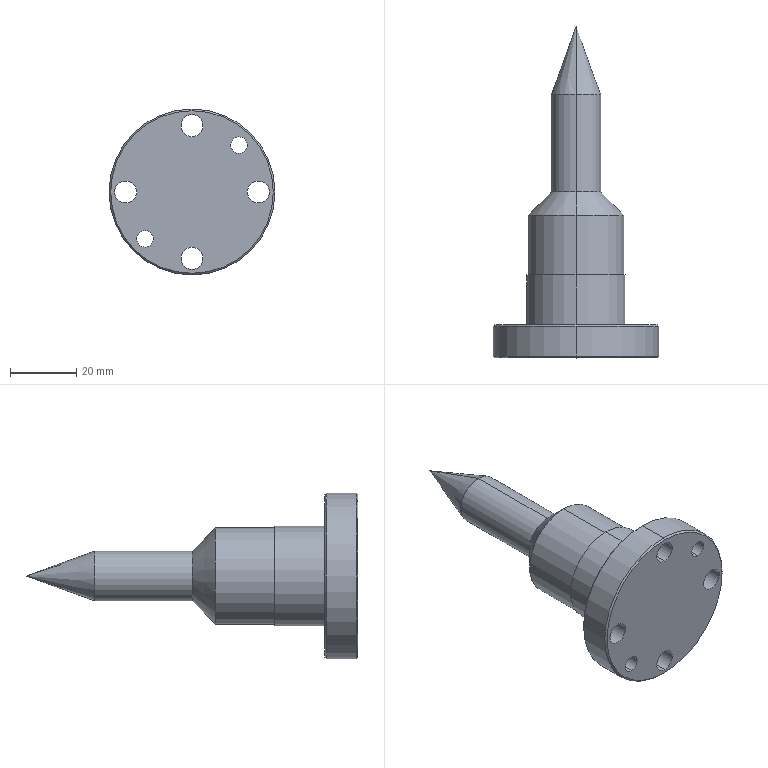Part | STEP file | HXGR200008-05-26 | 1 solid | 31 faces | box 50 x 100 x 50 mm | volume 49486 mm3 | cylinder 20 | cone 8 | plane 3 | commonest cylinder face diameters 6.6 x8 5 x4 15 x2 29 x2 30 x2 50 x2
STEP:
#1=CARTESIAN_POINT('',(0.,0.,-24.5));
#2=VERTEX_POINT('',#1);
#3=CARTESIAN_POINT('',(0.,0.,24.5));
#4=VERTEX_POINT('',#3);
#5=CARTESIAN_POINT('',(0.,0.,0.));
#6=DIRECTION('',(0.,-1.,0.));
#7=DIRECTION('',(0.,0.,1.));
#8=AXIS2_PLACEMENT_3D('',#5,#6,#7);
#9=CIRCLE('',#8,24.5);
#10=EDGE_CURVE('',#2,#4,#9,.T.);
#11=ORIENTED_EDGE('',*,*,#10,.F.);
#12=CARTESIAN_POINT('',(0.,0.5,-25.));
#13=VERTEX_POINT('',#12);
#14=CARTESIAN_POINT('',(0.,0.,-24.5));
#15=DIRECTION('',(0.,0.7071,-0.7071));
#16=VECTOR('',#15,1000.);
#17=LINE('',#14,#16);
#18=EDGE_CURVE('',#2,#13,#17,.T.);
#19=ORIENTED_EDGE('',*,*,#18,.T.);
#20=CARTESIAN_POINT('',(0.,0.5,25.));
#21=VERTEX_POINT('',#20);
#22=CARTESIAN_POINT('',(0.,0.5,0.));
#23=DIRECTION('',(0.,1.,0.));
#24=DIRECTION('',(0.,0.,1.));
#25=AXIS2_PLACEMENT_3D('',#22,#23,#24);
#26=CIRCLE('',#25,25.);
#27=EDGE_CURVE('',#21,#13,#26,.T.);
#28=ORIENTED_EDGE('',*,*,#27,.F.);
#29=CARTESIAN_POINT('',(0.,0.,24.5));
#30=DIRECTION('',(0.,0.7071,0.7071));
#31=VECTOR('',#30,1000.);
#32=LINE('',#29,#31);
#33=EDGE_CURVE('',#4,#21,#32,.T.);
#34=ORIENTED_EDGE('',*,*,#33,.F.);
#35=EDGE_LOOP('',(#11,#19,#28,#34));
#36=FACE_OUTER_BOUND('',#35,.T.);
#37=CARTESIAN_POINT('',(0.,0.,0.));
#38=DIRECTION('',(0.,1.,0.));
#39=DIRECTION('',(0.,0.,1.));
#40=AXIS2_PLACEMENT_3D('',#37,#38,#39);
#41=CONICAL_SURFACE('',#40,24.5,0.7854);
#42=ADVANCED_FACE('',(#36),#41,.T.);
#43=CARTESIAN_POINT('',(0.,10.,24.5));
#44=VERTEX_POINT('',#43);
#45=CARTESIAN_POINT('',(0.,10.,-24.5));
#46=VERTEX_POINT('',#45);
#47=CARTESIAN_POINT('',(0.,10.,0.));
#48=DIRECTION('',(0.,1.,0.));
#49=DIRECTION('',(0.,0.,-1.));
#50=AXIS2_PLACEMENT_3D('',#47,#48,#49);
#51=CIRCLE('',#50,24.5);
#52=EDGE_CURVE('',#44,#46,#51,.T.);
#53=ORIENTED_EDGE('',*,*,#52,.F.);
#54=CARTESIAN_POINT('',(0.,9.5,25.));
#55=VERTEX_POINT('',#54);
#56=CARTESIAN_POINT('',(0.,9.5,25.));
#57=DIRECTION('',(0.,-0.7071,0.7071));
#58=VECTOR('',#57,1000.);
#59=LINE('',#56,#58);
#60=EDGE_CURVE('',#44,#55,#59,.T.);
#61=ORIENTED_EDGE('',*,*,#60,.T.);
#62=CARTESIAN_POINT('',(0.,9.5,-25.));
#63=VERTEX_POINT('',#62);
#64=CARTESIAN_POINT('',(0.,9.5,0.));
#65=DIRECTION('',(0.,-1.,0.));
#66=DIRECTION('',(0.,0.,-1.));
#67=AXIS2_PLACEMENT_3D('',#64,#65,#66);
#68=CIRCLE('',#67,25.);
#69=EDGE_CURVE('',#63,#55,#68,.T.);
#70=ORIENTED_EDGE('',*,*,#69,.F.);
#71=CARTESIAN_POINT('',(0.,9.5,-25.));
#72=DIRECTION('',(0.,-0.7071,-0.7071));
#73=VECTOR('',#72,1000.);
#74=LINE('',#71,#73);
#75=EDGE_CURVE('',#46,#63,#74,.T.);
#76=ORIENTED_EDGE('',*,*,#75,.F.);
#77=EDGE_LOOP('',(#53,#61,#70,#76));
#78=FACE_OUTER_BOUND('',#77,.T.);
#79=CARTESIAN_POINT('',(0.,9.5,0.));
#80=DIRECTION('',(0.,-1.,0.));
#81=DIRECTION('',(0.,0.,-1.));
#82=AXIS2_PLACEMENT_3D('',#79,#80,#81);
#83=CONICAL_SURFACE('',#82,25.,0.7854);
#84=ADVANCED_FACE('',(#78),#83,.T.);
#85=CARTESIAN_POINT('',(0.,50.,-7.5));
#86=VERTEX_POINT('',#85);
#87=CARTESIAN_POINT('',(0.,50.,7.5));
#88=VERTEX_POINT('',#87);
#89=CARTESIAN_POINT('',(0.,50.,0.));
#90=DIRECTION('',(0.,-1.,0.));
#91=DIRECTION('',(0.,0.,-1.));
#92=AXIS2_PLACEMENT_3D('',#89,#90,#91);
#93=CIRCLE('',#92,7.5);
#94=EDGE_CURVE('',#86,#88,#93,.T.);
#95=ORIENTED_EDGE('',*,*,#94,.T.);
#96=CARTESIAN_POINT('',(0.,43.,14.5));
#97=VERTEX_POINT('',#96);
#98=CARTESIAN_POINT('',(0.,43.,14.5));
#99=DIRECTION('',(0.,-0.7071,0.7071));
#100=VECTOR('',#99,1000.);
#101=LINE('',#98,#100);
#102=EDGE_CURVE('',#88,#97,#101,.T.);
#103=ORIENTED_EDGE('',*,*,#102,.T.);
#104=CARTESIAN_POINT('',(0.,43.,-14.5));
#105=VERTEX_POINT('',#104);
#106=CARTESIAN_POINT('',(0.,43.,0.));
#107=DIRECTION('',(0.,-1.,0.));
#108=DIRECTION('',(0.,0.,-1.));
#109=AXIS2_PLACEMENT_3D('',#106,#107,#108);
#110=CIRCLE('',#109,14.5);
#111=EDGE_CURVE('',#105,#97,#110,.T.);
#112=ORIENTED_EDGE('',*,*,#111,.F.);
#113=CARTESIAN_POINT('',(0.,43.,-14.5));
#114=DIRECTION('',(0.,-0.7071,-0.7071));
#115=VECTOR('',#114,1000.);
#116=LINE('',#113,#115);
#117=EDGE_CURVE('',#86,#105,#116,.T.);
#118=ORIENTED_EDGE('',*,*,#117,.F.);
#119=EDGE_LOOP('',(#95,#103,#112,#118));
#120=FACE_OUTER_BOUND('',#119,.T.);
#121=CARTESIAN_POINT('',(0.,43.,0.));
#122=DIRECTION('',(0.,-1.,0.));
#123=DIRECTION('',(0.,0.,-1.));
#124=AXIS2_PLACEMENT_3D('',#121,#122,#123);
#125=CONICAL_SURFACE('',#124,14.5,0.7854);
#126=ADVANCED_FACE('',(#120),#125,.T.);
#127=CARTESIAN_POINT('',(14.142,0.,16.642));
#128=VERTEX_POINT('',#127);
#129=CARTESIAN_POINT('',(14.142,0.,11.642));
#130=VERTEX_POINT('',#129);
#131=CARTESIAN_POINT('',(14.142,0.,14.142));
#132=DIRECTION('',(0.,1.,0.));
#133=DIRECTION('',(0.,0.,-1.));
#134=AXIS2_PLACEMENT_3D('',#131,#132,#133);
#135=CIRCLE('',#134,2.5);
#136=EDGE_CURVE('',#128,#130,#135,.T.);
#137=ORIENTED_EDGE('',*,*,#136,.F.);
#138=CARTESIAN_POINT('',(14.142,10.,16.642));
#139=VERTEX_POINT('',#138);
#140=CARTESIAN_POINT('',(14.142,10.,16.642));
#141=DIRECTION('',(0.,1.,0.));
#142=VECTOR('',#141,1000.);
#143=LINE('',#140,#142);
#144=EDGE_CURVE('',#128,#139,#143,.T.);
#145=ORIENTED_EDGE('',*,*,#144,.T.);
#146=CARTESIAN_POINT('',(14.142,10.,11.642));
#147=VERTEX_POINT('',#146);
#148=CARTESIAN_POINT('',(14.142,10.,14.142));
#149=DIRECTION('',(0.,1.,0.));
#150=DIRECTION('',(0.,0.,-1.));
#151=AXIS2_PLACEMENT_3D('',#148,#149,#150);
#152=CIRCLE('',#151,2.5);
#153=EDGE_CURVE('',#139,#147,#152,.T.);
#154=ORIENTED_EDGE('',*,*,#153,.T.);
#155=CARTESIAN_POINT('',(14.142,10.,11.642));
#156=DIRECTION('',(0.,1.,0.));
#157=VECTOR('',#156,1000.);
#158=LINE('',#155,#157);
#159=EDGE_CURVE('',#130,#147,#158,.T.);
#160=ORIENTED_EDGE('',*,*,#159,.F.);
#161=EDGE_LOOP('',(#137,#145,#154,#160));
#162=FACE_OUTER_BOUND('',#161,.T.);
#163=CARTESIAN_POINT('',(14.142,10.,14.142));
#164=DIRECTION('',(0.,1.,0.));
#165=DIRECTION('',(0.,0.,-1.));
#166=AXIS2_PLACEMENT_3D('',#163,#164,#165);
#167=CYLINDRICAL_SURFACE('',#166,2.5);
#168=ADVANCED_FACE('',(#162),#167,.F.);
#169=CARTESIAN_POINT('',(-14.142,0.,-16.642));
#170=VERTEX_POINT('',#169);
#171=CARTESIAN_POINT('',(-14.142,0.,-11.642));
#172=VERTEX_POINT('',#171);
#173=CARTESIAN_POINT('',(-14.142,0.,-14.142));
#174=DIRECTION('',(0.,1.,0.));
#175=DIRECTION('',(0.,0.,1.));
#176=AXIS2_PLACEMENT_3D('',#173,#174,#175);
#177=CIRCLE('',#176,2.5);
#178=EDGE_CURVE('',#170,#172,#177,.T.);
#179=ORIENTED_EDGE('',*,*,#178,.F.);
#180=CARTESIAN_POINT('',(-14.142,10.,-16.642));
#181=VERTEX_POINT('',#180);
#182=CARTESIAN_POINT('',(-14.142,10.,-16.642));
#183=DIRECTION('',(0.,1.,0.));
#184=VECTOR('',#183,1000.);
#185=LINE('',#182,#184);
#186=EDGE_CURVE('',#170,#181,#185,.T.);
#187=ORIENTED_EDGE('',*,*,#186,.T.);
#188=CARTESIAN_POINT('',(-14.142,10.,-11.642));
#189=VERTEX_POINT('',#188);
#190=CARTESIAN_POINT('',(-14.142,10.,-14.142));
#191=DIRECTION('',(0.,1.,0.));
#192=DIRECTION('',(0.,0.,1.));
#193=AXIS2_PLACEMENT_3D('',#190,#191,#192);
#194=CIRCLE('',#193,2.5);
#195=EDGE_CURVE('',#181,#189,#194,.T.);
#196=ORIENTED_EDGE('',*,*,#195,.T.);
#197=CARTESIAN_POINT('',(-14.142,10.,-11.642));
#198=DIRECTION('',(0.,1.,0.));
#199=VECTOR('',#198,1000.);
#200=LINE('',#197,#199);
#201=EDGE_CURVE('',#172,#189,#200,.T.);
#202=ORIENTED_EDGE('',*,*,#201,.F.);
#203=EDGE_LOOP('',(#179,#187,#196,#202));
#204=FACE_OUTER_BOUND('',#203,.T.);
#205=CARTESIAN_POINT('',(-14.142,10.,-14.142));
#206=DIRECTION('',(0.,1.,0.));
#207=DIRECTION('',(0.,0.,1.));
#208=AXIS2_PLACEMENT_3D('',#205,#206,#207);
#209=CYLINDRICAL_SURFACE('',#208,2.5);
#210=ADVANCED_FACE('',(#204),#209,.F.);
#211=CARTESIAN_POINT('',(-23.3,0.,0.));
#212=VERTEX_POINT('',#211);
#213=CARTESIAN_POINT('',(-16.7,0.,0.));
#214=VERTEX_POINT('',#213);
#215=CARTESIAN_POINT('',(-20.,0.,0.));
#216=DIRECTION('',(0.,1.,0.));
#217=DIRECTION('',(1.,0.,0.));
#218=AXIS2_PLACEMENT_3D('',#215,#216,#217);
#219=CIRCLE('',#218,3.3);
#220=EDGE_CURVE('',#212,#214,#219,.T.);
#221=ORIENTED_EDGE('',*,*,#220,.F.);
#222=CARTESIAN_POINT('',(-23.3,10.,0.));
#223=VERTEX_POINT('',#222);
#224=CARTESIAN_POINT('',(-23.3,10.,0.));
#225=DIRECTION('',(0.,1.,0.));
#226=VECTOR('',#225,1000.);
#227=LINE('',#224,#226);
#228=EDGE_CURVE('',#212,#223,#227,.T.);
#229=ORIENTED_EDGE('',*,*,#228,.T.);
#230=CARTESIAN_POINT('',(-16.7,10.,0.));
#231=VERTEX_POINT('',#230);
#232=CARTESIAN_POINT('',(-20.,10.,0.));
#233=DIRECTION('',(0.,1.,0.));
#234=DIRECTION('',(1.,0.,0.));
#235=AXIS2_PLACEMENT_3D('',#232,#233,#234);
#236=CIRCLE('',#235,3.3);
#237=EDGE_CURVE('',#223,#231,#236,.T.);
#238=ORIENTED_EDGE('',*,*,#237,.T.);
#239=CARTESIAN_POINT('',(-16.7,10.,0.));
#240=DIRECTION('',(0.,1.,0.));
#241=VECTOR('',#240,1000.);
#242=LINE('',#239,#241);
#243=EDGE_CURVE('',#214,#231,#242,.T.);
#244=ORIENTED_EDGE('',*,*,#243,.F.);
#245=EDGE_LOOP('',(#221,#229,#238,#244));
#246=FACE_OUTER_BOUND('',#245,.T.);
#247=CARTESIAN_POINT('',(-20.,10.,0.));
#248=DIRECTION('',(0.,1.,0.));
#249=DIRECTION('',(1.,0.,0.));
#250=AXIS2_PLACEMENT_3D('',#247,#248,#249);
#251=CYLINDRICAL_SURFACE('',#250,3.3);
#252=ADVANCED_FACE('',(#246),#251,.F.);
#253=CARTESIAN_POINT('',(0.,0.,23.3));
#254=VERTEX_POINT('',#253);
#255=CARTESIAN_POINT('',(0.,0.,16.7));
#256=VERTEX_POINT('',#255);
#257=CARTESIAN_POINT('',(0.,0.,20.));
#258=DIRECTION('',(0.,1.,0.));
#259=DIRECTION('',(0.,0.,-1.));
#260=AXIS2_PLACEMENT_3D('',#257,#258,#259);
#261=CIRCLE('',#260,3.3);
#262=EDGE_CURVE('',#254,#256,#261,.T.);
#263=ORIENTED_EDGE('',*,*,#262,.F.);
#264=CARTESIAN_POINT('',(0.,10.,23.3));
#265=VERTEX_POINT('',#264);
#266=CARTESIAN_POINT('',(0.,10.,23.3));
#267=DIRECTION('',(0.,1.,0.));
#268=VECTOR('',#267,1000.);
#269=LINE('',#266,#268);
#270=EDGE_CURVE('',#254,#265,#269,.T.);
#271=ORIENTED_EDGE('',*,*,#270,.T.);
#272=CARTESIAN_POINT('',(0.,10.,16.7));
#273=VERTEX_POINT('',#272);
#274=CARTESIAN_POINT('',(0.,10.,20.));
#275=DIRECTION('',(0.,1.,0.));
#276=DIRECTION('',(0.,0.,-1.));
#277=AXIS2_PLACEMENT_3D('',#274,#275,#276);
#278=CIRCLE('',#277,3.3);
#279=EDGE_CURVE('',#265,#273,#278,.T.);
#280=ORIENTED_EDGE('',*,*,#279,.T.);
#281=CARTESIAN_POINT('',(0.,10.,16.7));
#282=DIRECTION('',(0.,1.,0.));
#283=VECTOR('',#282,1000.);
#284=LINE('',#281,#283);
#285=EDGE_CURVE('',#256,#273,#284,.T.);
#286=ORIENTED_EDGE('',*,*,#285,.F.);
#287=EDGE_LOOP('',(#263,#271,#280,#286));
#288=FACE_OUTER_BOUND('',#287,.T.);
#289=CARTESIAN_POINT('',(0.,10.,20.));
#290=DIRECTION('',(0.,1.,0.));
#291=DIRECTION('',(0.,0.,-1.));
#292=AXIS2_PLACEMENT_3D('',#289,#290,#291);
#293=CYLINDRICAL_SURFACE('',#292,3.3);
#294=ADVANCED_FACE('',(#288),#293,.F.);
#295=CARTESIAN_POINT('',(23.3,0.,0.));
#296=VERTEX_POINT('',#295);
#297=CARTESIAN_POINT('',(16.7,0.,0.));
#298=VERTEX_POINT('',#297);
#299=CARTESIAN_POINT('',(20.,0.,0.));
#300=DIRECTION('',(0.,1.,0.));
#301=DIRECTION('',(-1.,0.,0.));
#302=AXIS2_PLACEMENT_3D('',#299,#300,#301);
#303=CIRCLE('',#302,3.3);
#304=EDGE_CURVE('',#296,#298,#303,.T.);
#305=ORIENTED_EDGE('',*,*,#304,.F.);
#306=CARTESIAN_POINT('',(23.3,10.,0.));
#307=VERTEX_POINT('',#306);
#308=CARTESIAN_POINT('',(23.3,10.,0.));
#309=DIRECTION('',(0.,1.,0.));
#310=VECTOR('',#309,1000.);
#311=LINE('',#308,#310);
#312=EDGE_CURVE('',#296,#307,#311,.T.);
#313=ORIENTED_EDGE('',*,*,#312,.T.);
#314=CARTESIAN_POINT('',(16.7,10.,0.));
#315=VERTEX_POINT('',#314);
#316=CARTESIAN_POINT('',(20.,10.,0.));
#317=DIRECTION('',(0.,1.,0.));
#318=DIRECTION('',(-1.,0.,0.));
#319=AXIS2_PLACEMENT_3D('',#316,#317,#318);
#320=CIRCLE('',#319,3.3);
#321=EDGE_CURVE('',#307,#315,#320,.T.);
#322=ORIENTED_EDGE('',*,*,#321,.T.);
#323=CARTESIAN_POINT('',(16.7,10.,0.));
#324=DIRECTION('',(0.,1.,0.));
#325=VECTOR('',#324,1000.);
#326=LINE('',#323,#325);
#327=EDGE_CURVE('',#298,#315,#326,.T.);
#328=ORIENTED_EDGE('',*,*,#327,.F.);
#329=EDGE_LOOP('',(#305,#313,#322,#328));
#330=FACE_OUTER_BOUND('',#329,.T.);
#331=CARTESIAN_POINT('',(20.,10.,0.));
#332=DIRECTION('',(0.,1.,0.));
#333=DIRECTION('',(-1.,0.,0.));
#334=AXIS2_PLACEMENT_3D('',#331,#332,#333);
#335=CYLINDRICAL_SURFACE('',#334,3.3);
#336=ADVANCED_FACE('',(#330),#335,.F.);
#337=CARTESIAN_POINT('',(0.,0.,-23.3));
#338=VERTEX_POINT('',#337);
#339=CARTESIAN_POINT('',(0.,0.,-16.7));
#340=VERTEX_POINT('',#339);
#341=CARTESIAN_POINT('',(0.,0.,-20.));
#342=DIRECTION('',(0.,1.,0.));
#343=DIRECTION('',(0.,0.,1.));
#344=AXIS2_PLACEMENT_3D('',#341,#342,#343);
#345=CIRCLE('',#344,3.3);
#346=EDGE_CURVE('',#338,#340,#345,.T.);
#347=ORIENTED_EDGE('',*,*,#346,.F.);
#348=CARTESIAN_POINT('',(0.,10.,-23.3));
#349=VERTEX_POINT('',#348);
#350=CARTESIAN_POINT('',(0.,10.,-23.3));
#351=DIRECTION('',(0.,1.,0.));
#352=VECTOR('',#351,1000.);
#353=LINE('',#350,#352);
#354=EDGE_CURVE('',#338,#349,#353,.T.);
#355=ORIENTED_EDGE('',*,*,#354,.T.);
#356=CARTESIAN_POINT('',(0.,10.,-16.7));
#357=VERTEX_POINT('',#356);
#358=CARTESIAN_POINT('',(0.,10.,-20.));
#359=DIRECTION('',(0.,1.,0.));
#360=DIRECTION('',(0.,0.,1.));
#361=AXIS2_PLACEMENT_3D('',#358,#359,#360);
#362=CIRCLE('',#361,3.3);
#363=EDGE_CURVE('',#349,#357,#362,.T.);
#364=ORIENTED_EDGE('',*,*,#363,.T.);
#365=CARTESIAN_POINT('',(0.,10.,-16.7));
#366=DIRECTION('',(0.,1.,0.));
#367=VECTOR('',#366,1000.);
#368=LINE('',#365,#367);
#369=EDGE_CURVE('',#340,#357,#368,.T.);
#370=ORIENTED_EDGE('',*,*,#369,.F.);
#371=EDGE_LOOP('',(#347,#355,#364,#370));
#372=FACE_OUTER_BOUND('',#371,.T.);
#373=CARTESIAN_POINT('',(0.,10.,-20.));
#374=DIRECTION('',(0.,1.,0.));
#375=DIRECTION('',(0.,0.,1.));
#376=AXIS2_PLACEMENT_3D('',#373,#374,#375);
#377=CYLINDRICAL_SURFACE('',#376,3.3);
#378=ADVANCED_FACE('',(#372),#377,.F.);
#379=CARTESIAN_POINT('',(0.,100.,0.));
#380=VERTEX_POINT('',#379);
#381=CARTESIAN_POINT('',(0.,79.394,-7.5));
#382=VERTEX_POINT('',#381);
#383=CARTESIAN_POINT('',(0.,100.,0.));
#384=DIRECTION('',(0.,-0.9397,-0.342));
#385=VECTOR('',#384,1000.);
#386=LINE('',#383,#385);
#387=EDGE_CURVE('',#380,#382,#386,.T.);
#388=ORIENTED_EDGE('',*,*,#387,.F.);
#389=CARTESIAN_POINT('',(0.,79.394,7.5));
#390=VERTEX_POINT('',#389);
#391=CARTESIAN_POINT('',(0.,100.,0.));
#392=DIRECTION('',(0.,-0.9397,0.342));
#393=VECTOR('',#392,1000.);
#394=LINE('',#391,#393);
#395=EDGE_CURVE('',#380,#390,#394,.T.);
#396=ORIENTED_EDGE('',*,*,#395,.T.);
#397=CARTESIAN_POINT('',(0.,79.394,0.));
#398=DIRECTION('',(0.,-1.,0.));
#399=DIRECTION('',(0.,0.,-1.));
#400=AXIS2_PLACEMENT_3D('',#397,#398,#399);
#401=CIRCLE('',#400,7.5);
#402=EDGE_CURVE('',#382,#390,#401,.T.);
#403=ORIENTED_EDGE('',*,*,#402,.F.);
#404=EDGE_LOOP('',(#388,#396,#403));
#405=FACE_OUTER_BOUND('',#404,.T.);
#406=CARTESIAN_POINT('',(0.,-900.,0.));
#407=DIRECTION('',(0.,-1.,0.));
#408=DIRECTION('',(0.,0.,-1.));
#409=AXIS2_PLACEMENT_3D('',#406,#407,#408);
#410=CONICAL_SURFACE('',#409,363.97,0.3491);
#411=ADVANCED_FACE('',(#405),#410,.T.);
#412=ORIENTED_EDGE('',*,*,#402,.T.);
#413=CARTESIAN_POINT('',(0.,0.,7.5));
#414=DIRECTION('',(0.,-1.,0.));
#415=VECTOR('',#414,1000.);
#416=LINE('',#413,#415);
#417=EDGE_CURVE('',#390,#88,#416,.T.);
#418=ORIENTED_EDGE('',*,*,#417,.T.);
#419=ORIENTED_EDGE('',*,*,#94,.F.);
#420=CARTESIAN_POINT('',(0.,0.,-7.5));
#421=DIRECTION('',(0.,-1.,0.));
#422=VECTOR('',#421,1000.);
#423=LINE('',#420,#422);
#424=EDGE_CURVE('',#382,#86,#423,.T.);
#425=ORIENTED_EDGE('',*,*,#424,.F.);
#426=EDGE_LOOP('',(#412,#418,#419,#425));
#427=FACE_OUTER_BOUND('',#426,.T.);
#428=CARTESIAN_POINT('',(0.,0.,0.));
#429=DIRECTION('',(0.,-1.,0.));
#430=DIRECTION('',(0.,0.,-1.));
#431=AXIS2_PLACEMENT_3D('',#428,#429,#430);
#432=CYLINDRICAL_SURFACE('',#431,7.5);
#433=ADVANCED_FACE('',(#427),#432,.T.);
#434=ORIENTED_EDGE('',*,*,#111,.T.);
#435=CARTESIAN_POINT('',(0.,25.,14.5));
#436=VERTEX_POINT('',#435);
#437=CARTESIAN_POINT('',(0.,0.,14.5));
#438=DIRECTION('',(0.,-1.,0.));
#439=VECTOR('',#438,1000.);
#440=LINE('',#437,#439);
#441=EDGE_CURVE('',#97,#436,#440,.T.);
#442=ORIENTED_EDGE('',*,*,#441,.T.);
#443=CARTESIAN_POINT('',(0.,25.,-14.5));
#444=VERTEX_POINT('',#443);
#445=CARTESIAN_POINT('',(0.,25.,0.));
#446=DIRECTION('',(0.,-1.,0.));
#447=DIRECTION('',(0.,0.,-1.));
#448=AXIS2_PLACEMENT_3D('',#445,#446,#447);
#449=CIRCLE('',#448,14.5);
#450=EDGE_CURVE('',#444,#436,#449,.T.);
#451=ORIENTED_EDGE('',*,*,#450,.F.);
#452=CARTESIAN_POINT('',(0.,0.,-14.5));
#453=DIRECTION('',(0.,-1.,0.));
#454=VECTOR('',#453,1000.);
#455=LINE('',#452,#454);
#456=EDGE_CURVE('',#105,#444,#455,.T.);
#457=ORIENTED_EDGE('',*,*,#456,.F.);
#458=EDGE_LOOP('',(#434,#442,#451,#457));
#459=FACE_OUTER_BOUND('',#458,.T.);
#460=CARTESIAN_POINT('',(0.,0.,0.));
#461=DIRECTION('',(0.,-1.,0.));
#462=DIRECTION('',(0.,0.,-1.));
#463=AXIS2_PLACEMENT_3D('',#460,#461,#462);
#464=CYLINDRICAL_SURFACE('',#463,14.5);
#465=ADVANCED_FACE('',(#459),#464,.T.);
#466=CARTESIAN_POINT('',(0.,25.,-15.));
#467=VERTEX_POINT('',#466);
#468=CARTESIAN_POINT('',(0.,25.,15.));
#469=VERTEX_POINT('',#468);
#470=CARTESIAN_POINT('',(0.,25.,0.));
#471=DIRECTION('',(0.,-1.,0.));
#472=DIRECTION('',(0.,0.,-1.));
#473=AXIS2_PLACEMENT_3D('',#470,#471,#472);
#474=CIRCLE('',#473,15.);
#475=EDGE_CURVE('',#467,#469,#474,.T.);
#476=ORIENTED_EDGE('',*,*,#475,.T.);
#477=CARTESIAN_POINT('',(0.,10.,15.));
#478=VERTEX_POINT('',#477);
#479=CARTESIAN_POINT('',(0.,0.,15.));
#480=DIRECTION('',(0.,-1.,0.));
#481=VECTOR('',#480,1000.);
#482=LINE('',#479,#481);
#483=EDGE_CURVE('',#469,#478,#482,.T.);
#484=ORIENTED_EDGE('',*,*,#483,.T.);
#485=CARTESIAN_POINT('',(0.,10.,-15.));
#486=VERTEX_POINT('',#485);
#487=CARTESIAN_POINT('',(0.,10.,0.));
#488=DIRECTION('',(0.,-1.,0.));
#489=DIRECTION('',(0.,0.,-1.));
#490=AXIS2_PLACEMENT_3D('',#487,#488,#489);
#491=CIRCLE('',#490,15.);
#492=EDGE_CURVE('',#486,#478,#491,.T.);
#493=ORIENTED_EDGE('',*,*,#492,.F.);
#494=CARTESIAN_POINT('',(0.,0.,-15.));
#495=DIRECTION('',(0.,-1.,0.));
#496=VECTOR('',#495,1000.);
#497=LINE('',#494,#496);
#498=EDGE_CURVE('',#467,#486,#497,.T.);
#499=ORIENTED_EDGE('',*,*,#498,.F.);
#500=EDGE_LOOP('',(#476,#484,#493,#499));
#501=FACE_OUTER_BOUND('',#500,.T.);
#502=CARTESIAN_POINT('',(0.,0.,0.));
#503=DIRECTION('',(0.,-1.,0.));
#504=DIRECTION('',(0.,0.,-1.));
#505=AXIS2_PLACEMENT_3D('',#502,#503,#504);
#506=CYLINDRICAL_SURFACE('',#505,15.);
#507=ADVANCED_FACE('',(#501),#506,.T.);
#508=ORIENTED_EDGE('',*,*,#69,.T.);
#509=CARTESIAN_POINT('',(0.,0.,25.));
#510=DIRECTION('',(0.,-1.,0.));
#511=VECTOR('',#510,1000.);
#512=LINE('',#509,#511);
#513=EDGE_CURVE('',#55,#21,#512,.T.);
#514=ORIENTED_EDGE('',*,*,#513,.T.);
#515=ORIENTED_EDGE('',*,*,#27,.T.);
#516=CARTESIAN_POINT('',(0.,0.,-25.));
#517=DIRECTION('',(0.,-1.,0.));
#518=VECTOR('',#517,1000.);
#519=LINE('',#516,#518);
#520=EDGE_CURVE('',#63,#13,#519,.T.);
#521=ORIENTED_EDGE('',*,*,#520,.F.);
#522=EDGE_LOOP('',(#508,#514,#515,#521));
#523=FACE_OUTER_BOUND('',#522,.T.);
#524=CARTESIAN_POINT('',(0.,0.,0.));
#525=DIRECTION('',(0.,-1.,0.));
#526=DIRECTION('',(0.,0.,-1.));
#527=AXIS2_PLACEMENT_3D('',#524,#525,#526);
#528=CYLINDRICAL_SURFACE('',#527,25.);
#529=ADVANCED_FACE('',(#523),#528,.T.);
#530=CARTESIAN_POINT('',(0.,10.,0.));
#531=DIRECTION('',(0.,1.,0.));
#532=DIRECTION('',(0.,0.,-1.));
#533=AXIS2_PLACEMENT_3D('',#530,#531,#532);
#534=CIRCLE('',#533,24.5);
#535=EDGE_CURVE('',#46,#44,#534,.T.);
#536=ORIENTED_EDGE('',*,*,#535,.T.);
#537=ORIENTED_EDGE('',*,*,#52,.T.);
#538=EDGE_LOOP('',(#536,#537));
#539=FACE_OUTER_BOUND('',#538,.T.);
#540=CARTESIAN_POINT('',(14.142,10.,14.142));
#541=DIRECTION('',(0.,1.,0.));
#542=DIRECTION('',(0.,0.,-1.));
#543=AXIS2_PLACEMENT_3D('',#540,#541,#542);
#544=CIRCLE('',#543,2.5);
#545=EDGE_CURVE('',#147,#139,#544,.T.);
#546=ORIENTED_EDGE('',*,*,#545,.F.);
#547=ORIENTED_EDGE('',*,*,#153,.F.);
#548=EDGE_LOOP('',(#546,#547));
#549=FACE_BOUND('',#548,.T.);
#550=CARTESIAN_POINT('',(-20.,10.,0.));
#551=DIRECTION('',(0.,1.,0.));
#552=DIRECTION('',(1.,0.,0.));
#553=AXIS2_PLACEMENT_3D('',#550,#551,#552);
#554=CIRCLE('',#553,3.3);
#555=EDGE_CURVE('',#231,#223,#554,.T.);
#556=ORIENTED_EDGE('',*,*,#555,.F.);
#557=ORIENTED_EDGE('',*,*,#237,.F.);
#558=EDGE_LOOP('',(#556,#557));
#559=FACE_BOUND('',#558,.T.);
#560=CARTESIAN_POINT('',(0.,10.,20.));
#561=DIRECTION('',(0.,1.,0.));
#562=DIRECTION('',(0.,0.,-1.));
#563=AXIS2_PLACEMENT_3D('',#560,#561,#562);
#564=CIRCLE('',#563,3.3);
#565=EDGE_CURVE('',#273,#265,#564,.T.);
#566=ORIENTED_EDGE('',*,*,#565,.F.);
#567=ORIENTED_EDGE('',*,*,#279,.F.);
#568=EDGE_LOOP('',(#566,#567));
#569=FACE_BOUND('',#568,.T.);
#570=CARTESIAN_POINT('',(20.,10.,0.));
#571=DIRECTION('',(0.,1.,0.));
#572=DIRECTION('',(-1.,0.,0.));
#573=AXIS2_PLACEMENT_3D('',#570,#571,#572);
#574=CIRCLE('',#573,3.3);
#575=EDGE_CURVE('',#315,#307,#574,.T.);
#576=ORIENTED_EDGE('',*,*,#575,.F.);
#577=ORIENTED_EDGE('',*,*,#321,.F.);
#578=EDGE_LOOP('',(#576,#577));
#579=FACE_BOUND('',#578,.T.);
#580=ORIENTED_EDGE('',*,*,#492,.T.);
#581=CARTESIAN_POINT('',(0.,10.,0.));
#582=DIRECTION('',(0.,-1.,0.));
#583=DIRECTION('',(0.,0.,-1.));
#584=AXIS2_PLACEMENT_3D('',#581,#582,#583);
#585=CIRCLE('',#584,15.);
#586=EDGE_CURVE('',#478,#486,#585,.T.);
#587=ORIENTED_EDGE('',*,*,#586,.T.);
#588=EDGE_LOOP('',(#580,#587));
#589=FACE_BOUND('',#588,.T.);
#590=CARTESIAN_POINT('',(0.,10.,-20.));
#591=DIRECTION('',(0.,1.,0.));
#592=DIRECTION('',(0.,0.,1.));
#593=AXIS2_PLACEMENT_3D('',#590,#591,#592);
#594=CIRCLE('',#593,3.3);
#595=EDGE_CURVE('',#357,#349,#594,.T.);
#596=ORIENTED_EDGE('',*,*,#595,.F.);
#597=ORIENTED_EDGE('',*,*,#363,.F.);
#598=EDGE_LOOP('',(#596,#597));
#599=FACE_BOUND('',#598,.T.);
#600=CARTESIAN_POINT('',(-14.142,10.,-14.142));
#601=DIRECTION('',(0.,1.,0.));
#602=DIRECTION('',(0.,0.,1.));
#603=AXIS2_PLACEMENT_3D('',#600,#601,#602);
#604=CIRCLE('',#603,2.5);
#605=EDGE_CURVE('',#189,#181,#604,.T.);
#606=ORIENTED_EDGE('',*,*,#605,.F.);
#607=ORIENTED_EDGE('',*,*,#195,.F.);
#608=EDGE_LOOP('',(#606,#607));
#609=FACE_BOUND('',#608,.T.);
#610=CARTESIAN_POINT('',(-25.,10.,0.));
#611=DIRECTION('',(0.,-1.,0.));
#612=DIRECTION('',(0.,0.,-1.));
#613=AXIS2_PLACEMENT_3D('',#610,#611,#612);
#614=PLANE('',#613);
#615=ADVANCED_FACE('',(#539,#549,#559,#569,#579,#589,#599,#609),#614,.F.);
#616=CARTESIAN_POINT('',(0.,0.,0.));
#617=DIRECTION('',(0.,-1.,0.));
#618=DIRECTION('',(0.,0.,1.));
#619=AXIS2_PLACEMENT_3D('',#616,#617,#618);
#620=CIRCLE('',#619,24.5);
#621=EDGE_CURVE('',#4,#2,#620,.T.);
#622=ORIENTED_EDGE('',*,*,#621,.T.);
#623=ORIENTED_EDGE('',*,*,#10,.T.);
#624=EDGE_LOOP('',(#622,#623));
#625=FACE_OUTER_BOUND('',#624,.T.);
#626=CARTESIAN_POINT('',(14.142,0.,14.142));
#627=DIRECTION('',(0.,1.,0.));
#628=DIRECTION('',(0.,0.,-1.));
#629=AXIS2_PLACEMENT_3D('',#626,#627,#628);
#630=CIRCLE('',#629,2.5);
#631=EDGE_CURVE('',#130,#128,#630,.T.);
#632=ORIENTED_EDGE('',*,*,#631,.T.);
#633=ORIENTED_EDGE('',*,*,#136,.T.);
#634=EDGE_LOOP('',(#632,#633));
#635=FACE_BOUND('',#634,.T.);
#636=CARTESIAN_POINT('',(-14.142,0.,-14.142));
#637=DIRECTION('',(0.,1.,0.));
#638=DIRECTION('',(0.,0.,1.));
#639=AXIS2_PLACEMENT_3D('',#636,#637,#638);
#640=CIRCLE('',#639,2.5);
#641=EDGE_CURVE('',#172,#170,#640,.T.);
#642=ORIENTED_EDGE('',*,*,#641,.T.);
#643=ORIENTED_EDGE('',*,*,#178,.T.);
#644=EDGE_LOOP('',(#642,#643));
#645=FACE_BOUND('',#644,.T.);
#646=CARTESIAN_POINT('',(-20.,0.,0.));
#647=DIRECTION('',(0.,1.,0.));
#648=DIRECTION('',(1.,0.,0.));
#649=AXIS2_PLACEMENT_3D('',#646,#647,#648);
#650=CIRCLE('',#649,3.3);
#651=EDGE_CURVE('',#214,#212,#650,.T.);
#652=ORIENTED_EDGE('',*,*,#651,.T.);
#653=ORIENTED_EDGE('',*,*,#220,.T.);
#654=EDGE_LOOP('',(#652,#653));
#655=FACE_BOUND('',#654,.T.);
#656=CARTESIAN_POINT('',(0.,0.,20.));
#657=DIRECTION('',(0.,1.,0.));
#658=DIRECTION('',(0.,0.,-1.));
#659=AXIS2_PLACEMENT_3D('',#656,#657,#658);
#660=CIRCLE('',#659,3.3);
#661=EDGE_CURVE('',#256,#254,#660,.T.);
#662=ORIENTED_EDGE('',*,*,#661,.T.);
#663=ORIENTED_EDGE('',*,*,#262,.T.);
#664=EDGE_LOOP('',(#662,#663));
#665=FACE_BOUND('',#664,.T.);
#666=CARTESIAN_POINT('',(20.,0.,0.));
#667=DIRECTION('',(0.,1.,0.));
#668=DIRECTION('',(-1.,0.,0.));
#669=AXIS2_PLACEMENT_3D('',#666,#667,#668);
#670=CIRCLE('',#669,3.3);
#671=EDGE_CURVE('',#298,#296,#670,.T.);
#672=ORIENTED_EDGE('',*,*,#671,.T.);
#673=ORIENTED_EDGE('',*,*,#304,.T.);
#674=EDGE_LOOP('',(#672,#673));
#675=FACE_BOUND('',#674,.T.);
#676=CARTESIAN_POINT('',(0.,0.,-20.));
#677=DIRECTION('',(0.,1.,0.));
#678=DIRECTION('',(0.,0.,1.));
#679=AXIS2_PLACEMENT_3D('',#676,#677,#678);
#680=CIRCLE('',#679,3.3);
#681=EDGE_CURVE('',#340,#338,#680,.T.);
#682=ORIENTED_EDGE('',*,*,#681,.T.);
#683=ORIENTED_EDGE('',*,*,#346,.T.);
#684=EDGE_LOOP('',(#682,#683));
#685=FACE_BOUND('',#684,.T.);
#686=CARTESIAN_POINT('',(0.,0.,0.));
#687=DIRECTION('',(0.,1.,0.));
#688=DIRECTION('',(0.,0.,1.));
#689=AXIS2_PLACEMENT_3D('',#686,#687,#688);
#690=PLANE('',#689);
#691=ADVANCED_FACE('',(#625,#635,#645,#655,#665,#675,#685),#690,.F.);
#692=ORIENTED_EDGE('',*,*,#513,.F.);
#693=CARTESIAN_POINT('',(0.,9.5,0.));
#694=DIRECTION('',(0.,-1.,0.));
#695=DIRECTION('',(0.,0.,-1.));
#696=AXIS2_PLACEMENT_3D('',#693,#694,#695);
#697=CIRCLE('',#696,25.);
#698=EDGE_CURVE('',#55,#63,#697,.T.);
#699=ORIENTED_EDGE('',*,*,#698,.T.);
#700=ORIENTED_EDGE('',*,*,#520,.T.);
#701=CARTESIAN_POINT('',(0.,0.5,0.));
#702=DIRECTION('',(0.,1.,0.));
#703=DIRECTION('',(0.,0.,1.));
#704=AXIS2_PLACEMENT_3D('',#701,#702,#703);
#705=CIRCLE('',#704,25.);
#706=EDGE_CURVE('',#13,#21,#705,.T.);
#707=ORIENTED_EDGE('',*,*,#706,.T.);
#708=EDGE_LOOP('',(#692,#699,#700,#707));
#709=FACE_OUTER_BOUND('',#708,.T.);
#710=CARTESIAN_POINT('',(0.,0.,0.));
#711=DIRECTION('',(0.,-1.,0.));
#712=DIRECTION('',(0.,0.,-1.));
#713=AXIS2_PLACEMENT_3D('',#710,#711,#712);
#714=CYLINDRICAL_SURFACE('',#713,25.);
#715=ADVANCED_FACE('',(#709),#714,.T.);
#716=ORIENTED_EDGE('',*,*,#483,.F.);
#717=CARTESIAN_POINT('',(0.,25.,0.));
#718=DIRECTION('',(0.,-1.,0.));
#719=DIRECTION('',(0.,0.,-1.));
#720=AXIS2_PLACEMENT_3D('',#717,#718,#719);
#721=CIRCLE('',#720,15.);
#722=EDGE_CURVE('',#469,#467,#721,.T.);
#723=ORIENTED_EDGE('',*,*,#722,.T.);
#724=ORIENTED_EDGE('',*,*,#498,.T.);
#725=ORIENTED_EDGE('',*,*,#586,.F.);
#726=EDGE_LOOP('',(#716,#723,#724,#725));
#727=FACE_OUTER_BOUND('',#726,.T.);
#728=CARTESIAN_POINT('',(0.,0.,0.));
#729=DIRECTION('',(0.,-1.,0.));
#730=DIRECTION('',(0.,0.,-1.));
#731=AXIS2_PLACEMENT_3D('',#728,#729,#730);
#732=CYLINDRICAL_SURFACE('',#731,15.);
#733=ADVANCED_FACE('',(#727),#732,.T.);
#734=ORIENTED_EDGE('',*,*,#475,.F.);
#735=ORIENTED_EDGE('',*,*,#722,.F.);
#736=EDGE_LOOP('',(#734,#735));
#737=FACE_OUTER_BOUND('',#736,.T.);
#738=ORIENTED_EDGE('',*,*,#450,.T.);
#739=CARTESIAN_POINT('',(0.,25.,0.));
#740=DIRECTION('',(0.,-1.,0.));
#741=DIRECTION('',(0.,0.,-1.));
#742=AXIS2_PLACEMENT_3D('',#739,#740,#741);
#743=CIRCLE('',#742,14.5);
#744=EDGE_CURVE('',#436,#444,#743,.T.);
#745=ORIENTED_EDGE('',*,*,#744,.T.);
#746=EDGE_LOOP('',(#738,#745));
#747=FACE_BOUND('',#746,.T.);
#748=CARTESIAN_POINT('',(-14.5,25.,0.));
#749=DIRECTION('',(0.,-1.,0.));
#750=DIRECTION('',(0.,0.,-1.));
#751=AXIS2_PLACEMENT_3D('',#748,#749,#750);
#752=PLANE('',#751);
#753=ADVANCED_FACE('',(#737,#747),#752,.F.);
#754=ORIENTED_EDGE('',*,*,#441,.F.);
#755=CARTESIAN_POINT('',(0.,43.,0.));
#756=DIRECTION('',(0.,-1.,0.));
#757=DIRECTION('',(0.,0.,-1.));
#758=AXIS2_PLACEMENT_3D('',#755,#756,#757);
#759=CIRCLE('',#758,14.5);
#760=EDGE_CURVE('',#97,#105,#759,.T.);
#761=ORIENTED_EDGE('',*,*,#760,.T.);
#762=ORIENTED_EDGE('',*,*,#456,.T.);
#763=ORIENTED_EDGE('',*,*,#744,.F.);
#764=EDGE_LOOP('',(#754,#761,#762,#763));
#765=FACE_OUTER_BOUND('',#764,.T.);
#766=CARTESIAN_POINT('',(0.,0.,0.));
#767=DIRECTION('',(0.,-1.,0.));
#768=DIRECTION('',(0.,0.,-1.));
#769=AXIS2_PLACEMENT_3D('',#766,#767,#768);
#770=CYLINDRICAL_SURFACE('',#769,14.5);
#771=ADVANCED_FACE('',(#765),#770,.T.);
#772=ORIENTED_EDGE('',*,*,#417,.F.);
#773=CARTESIAN_POINT('',(0.,79.394,0.));
#774=DIRECTION('',(0.,-1.,0.));
#775=DIRECTION('',(0.,0.,-1.));
#776=AXIS2_PLACEMENT_3D('',#773,#774,#775);
#777=CIRCLE('',#776,7.5);
#778=EDGE_CURVE('',#390,#382,#777,.T.);
#779=ORIENTED_EDGE('',*,*,#778,.T.);
#780=ORIENTED_EDGE('',*,*,#424,.T.);
#781=CARTESIAN_POINT('',(0.,50.,0.));
#782=DIRECTION('',(0.,-1.,0.));
#783=DIRECTION('',(0.,0.,-1.));
#784=AXIS2_PLACEMENT_3D('',#781,#782,#783);
#785=CIRCLE('',#784,7.5);
#786=EDGE_CURVE('',#88,#86,#785,.T.);
#787=ORIENTED_EDGE('',*,*,#786,.F.);
#788=EDGE_LOOP('',(#772,#779,#780,#787));
#789=FACE_OUTER_BOUND('',#788,.T.);
#790=CARTESIAN_POINT('',(0.,0.,0.));
#791=DIRECTION('',(0.,-1.,0.));
#792=DIRECTION('',(0.,0.,-1.));
#793=AXIS2_PLACEMENT_3D('',#790,#791,#792);
#794=CYLINDRICAL_SURFACE('',#793,7.5);
#795=ADVANCED_FACE('',(#789),#794,.T.);
#796=ORIENTED_EDGE('',*,*,#395,.F.);
#797=ORIENTED_EDGE('',*,*,#387,.T.);
#798=ORIENTED_EDGE('',*,*,#778,.F.);
#799=EDGE_LOOP('',(#796,#797,#798));
#800=FACE_OUTER_BOUND('',#799,.T.);
#801=CARTESIAN_POINT('',(0.,-900.,0.));
#802=DIRECTION('',(0.,-1.,0.));
#803=DIRECTION('',(0.,0.,-1.));
#804=AXIS2_PLACEMENT_3D('',#801,#802,#803);
#805=CONICAL_SURFACE('',#804,363.97,0.3491);
#806=ADVANCED_FACE('',(#800),#805,.T.);
#807=ORIENTED_EDGE('',*,*,#354,.F.);
#808=ORIENTED_EDGE('',*,*,#681,.F.);
#809=ORIENTED_EDGE('',*,*,#369,.T.);
#810=ORIENTED_EDGE('',*,*,#595,.T.);
#811=EDGE_LOOP('',(#807,#808,#809,#810));
#812=FACE_OUTER_BOUND('',#811,.T.);
#813=CARTESIAN_POINT('',(0.,10.,-20.));
#814=DIRECTION('',(0.,1.,0.));
#815=DIRECTION('',(0.,0.,1.));
#816=AXIS2_PLACEMENT_3D('',#813,#814,#815);
#817=CYLINDRICAL_SURFACE('',#816,3.3);
#818=ADVANCED_FACE('',(#812),#817,.F.);
#819=ORIENTED_EDGE('',*,*,#312,.F.);
#820=ORIENTED_EDGE('',*,*,#671,.F.);
#821=ORIENTED_EDGE('',*,*,#327,.T.);
#822=ORIENTED_EDGE('',*,*,#575,.T.);
#823=EDGE_LOOP('',(#819,#820,#821,#822));
#824=FACE_OUTER_BOUND('',#823,.T.);
#825=CARTESIAN_POINT('',(20.,10.,0.));
#826=DIRECTION('',(0.,1.,0.));
#827=DIRECTION('',(-1.,0.,0.));
#828=AXIS2_PLACEMENT_3D('',#825,#826,#827);
#829=CYLINDRICAL_SURFACE('',#828,3.3);
#830=ADVANCED_FACE('',(#824),#829,.F.);
#831=ORIENTED_EDGE('',*,*,#270,.F.);
#832=ORIENTED_EDGE('',*,*,#661,.F.);
#833=ORIENTED_EDGE('',*,*,#285,.T.);
#834=ORIENTED_EDGE('',*,*,#565,.T.);
#835=EDGE_LOOP('',(#831,#832,#833,#834));
#836=FACE_OUTER_BOUND('',#835,.T.);
#837=CARTESIAN_POINT('',(0.,10.,20.));
#838=DIRECTION('',(0.,1.,0.));
#839=DIRECTION('',(0.,0.,-1.));
#840=AXIS2_PLACEMENT_3D('',#837,#838,#839);
#841=CYLINDRICAL_SURFACE('',#840,3.3);
#842=ADVANCED_FACE('',(#836),#841,.F.);
#843=ORIENTED_EDGE('',*,*,#228,.F.);
#844=ORIENTED_EDGE('',*,*,#651,.F.);
#845=ORIENTED_EDGE('',*,*,#243,.T.);
#846=ORIENTED_EDGE('',*,*,#555,.T.);
#847=EDGE_LOOP('',(#843,#844,#845,#846));
#848=FACE_OUTER_BOUND('',#847,.T.);
#849=CARTESIAN_POINT('',(-20.,10.,0.));
#850=DIRECTION('',(0.,1.,0.));
#851=DIRECTION('',(1.,0.,0.));
#852=AXIS2_PLACEMENT_3D('',#849,#850,#851);
#853=CYLINDRICAL_SURFACE('',#852,3.3);
#854=ADVANCED_FACE('',(#848),#853,.F.);
#855=ORIENTED_EDGE('',*,*,#186,.F.);
#856=ORIENTED_EDGE('',*,*,#641,.F.);
#857=ORIENTED_EDGE('',*,*,#201,.T.);
#858=ORIENTED_EDGE('',*,*,#605,.T.);
#859=EDGE_LOOP('',(#855,#856,#857,#858));
#860=FACE_OUTER_BOUND('',#859,.T.);
#861=CARTESIAN_POINT('',(-14.142,10.,-14.142));
#862=DIRECTION('',(0.,1.,0.));
#863=DIRECTION('',(0.,0.,1.));
#864=AXIS2_PLACEMENT_3D('',#861,#862,#863);
#865=CYLINDRICAL_SURFACE('',#864,2.5);
#866=ADVANCED_FACE('',(#860),#865,.F.);
#867=ORIENTED_EDGE('',*,*,#144,.F.);
#868=ORIENTED_EDGE('',*,*,#631,.F.);
#869=ORIENTED_EDGE('',*,*,#159,.T.);
#870=ORIENTED_EDGE('',*,*,#545,.T.);
#871=EDGE_LOOP('',(#867,#868,#869,#870));
#872=FACE_OUTER_BOUND('',#871,.T.);
#873=CARTESIAN_POINT('',(14.142,10.,14.142));
#874=DIRECTION('',(0.,1.,0.));
#875=DIRECTION('',(0.,0.,-1.));
#876=AXIS2_PLACEMENT_3D('',#873,#874,#875);
#877=CYLINDRICAL_SURFACE('',#876,2.5);
#878=ADVANCED_FACE('',(#872),#877,.F.);
#879=ORIENTED_EDGE('',*,*,#102,.F.);
#880=ORIENTED_EDGE('',*,*,#786,.T.);
#881=ORIENTED_EDGE('',*,*,#117,.T.);
#882=ORIENTED_EDGE('',*,*,#760,.F.);
#883=EDGE_LOOP('',(#879,#880,#881,#882));
#884=FACE_OUTER_BOUND('',#883,.T.);
#885=CARTESIAN_POINT('',(0.,43.,0.));
#886=DIRECTION('',(0.,-1.,0.));
#887=DIRECTION('',(0.,0.,-1.));
#888=AXIS2_PLACEMENT_3D('',#885,#886,#887);
#889=CONICAL_SURFACE('',#888,14.5,0.7854);
#890=ADVANCED_FACE('',(#884),#889,.T.);
#891=ORIENTED_EDGE('',*,*,#60,.F.);
#892=ORIENTED_EDGE('',*,*,#535,.F.);
#893=ORIENTED_EDGE('',*,*,#75,.T.);
#894=ORIENTED_EDGE('',*,*,#698,.F.);
#895=EDGE_LOOP('',(#891,#892,#893,#894));
#896=FACE_OUTER_BOUND('',#895,.T.);
#897=CARTESIAN_POINT('',(0.,9.5,0.));
#898=DIRECTION('',(0.,-1.,0.));
#899=DIRECTION('',(0.,0.,-1.));
#900=AXIS2_PLACEMENT_3D('',#897,#898,#899);
#901=CONICAL_SURFACE('',#900,25.,0.7854);
#902=ADVANCED_FACE('',(#896),#901,.T.);
#903=ORIENTED_EDGE('',*,*,#18,.F.);
#904=ORIENTED_EDGE('',*,*,#621,.F.);
#905=ORIENTED_EDGE('',*,*,#33,.T.);
#906=ORIENTED_EDGE('',*,*,#706,.F.);
#907=EDGE_LOOP('',(#903,#904,#905,#906));
#908=FACE_OUTER_BOUND('',#907,.T.);
#909=CARTESIAN_POINT('',(0.,0.,0.));
#910=DIRECTION('',(0.,1.,0.));
#911=DIRECTION('',(0.,0.,1.));
#912=AXIS2_PLACEMENT_3D('',#909,#910,#911);
#913=CONICAL_SURFACE('',#912,24.5,0.7854);
#914=ADVANCED_FACE('',(#908),#913,.T.);
#915=CLOSED_SHELL('',(#42,#84,#126,#168,#210,#252,#294,#336,#378,#411,#433,#465,#507,#529,#615,#691,#715,#733,#753,#771,#795,#806,#818,#830,#842,#854,#866,#878,#890,#902,#914));
#916=MANIFOLD_SOLID_BREP('',#915);
#917=CARTESIAN_POINT('',(0.,0.,0.));
#918=DIRECTION('',(0.,0.,1.));
#919=DIRECTION('',(1.,0.,0.));
#920=AXIS2_PLACEMENT_3D('',#917,#918,#919);
#921=(LENGTH_UNIT()NAMED_UNIT(*)SI_UNIT(.MILLI.,.METRE.));
#922=UNCERTAINTY_MEASURE_WITH_UNIT(LENGTH_MEASURE(0.00001),#921,'','');
#923=(NAMED_UNIT(*)PLANE_ANGLE_UNIT()SI_UNIT($,.RADIAN.));
#924=(NAMED_UNIT(*)SI_UNIT($,.STERADIAN.)SOLID_ANGLE_UNIT());
#925=(GEOMETRIC_REPRESENTATION_CONTEXT(3)GLOBAL_UNCERTAINTY_ASSIGNED_CONTEXT((#922))GLOBAL_UNIT_ASSIGNED_CONTEXT((#921,#923,#924))REPRESENTATION_CONTEXT('',''));
#926=ADVANCED_BREP_SHAPE_REPRESENTATION('',(#916,#920),#925);